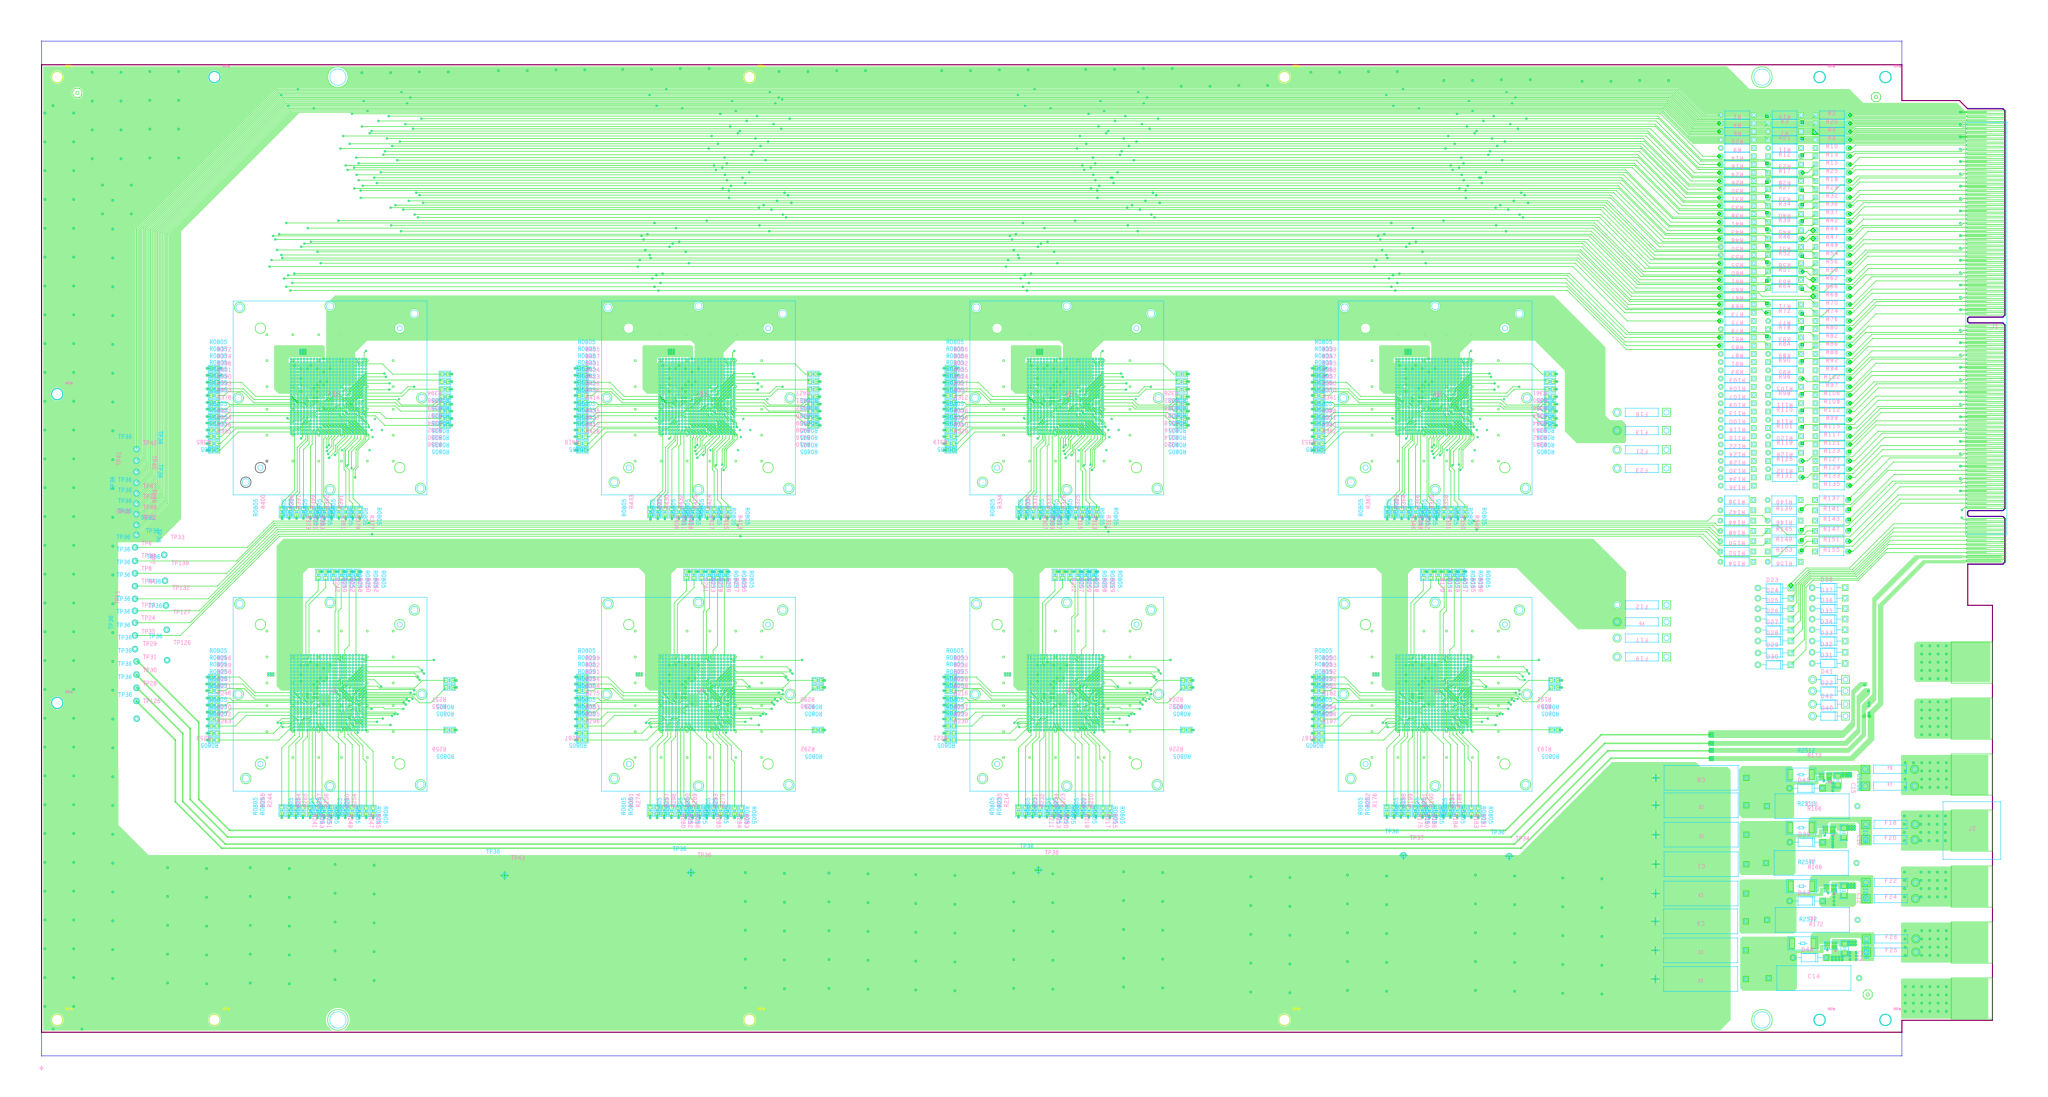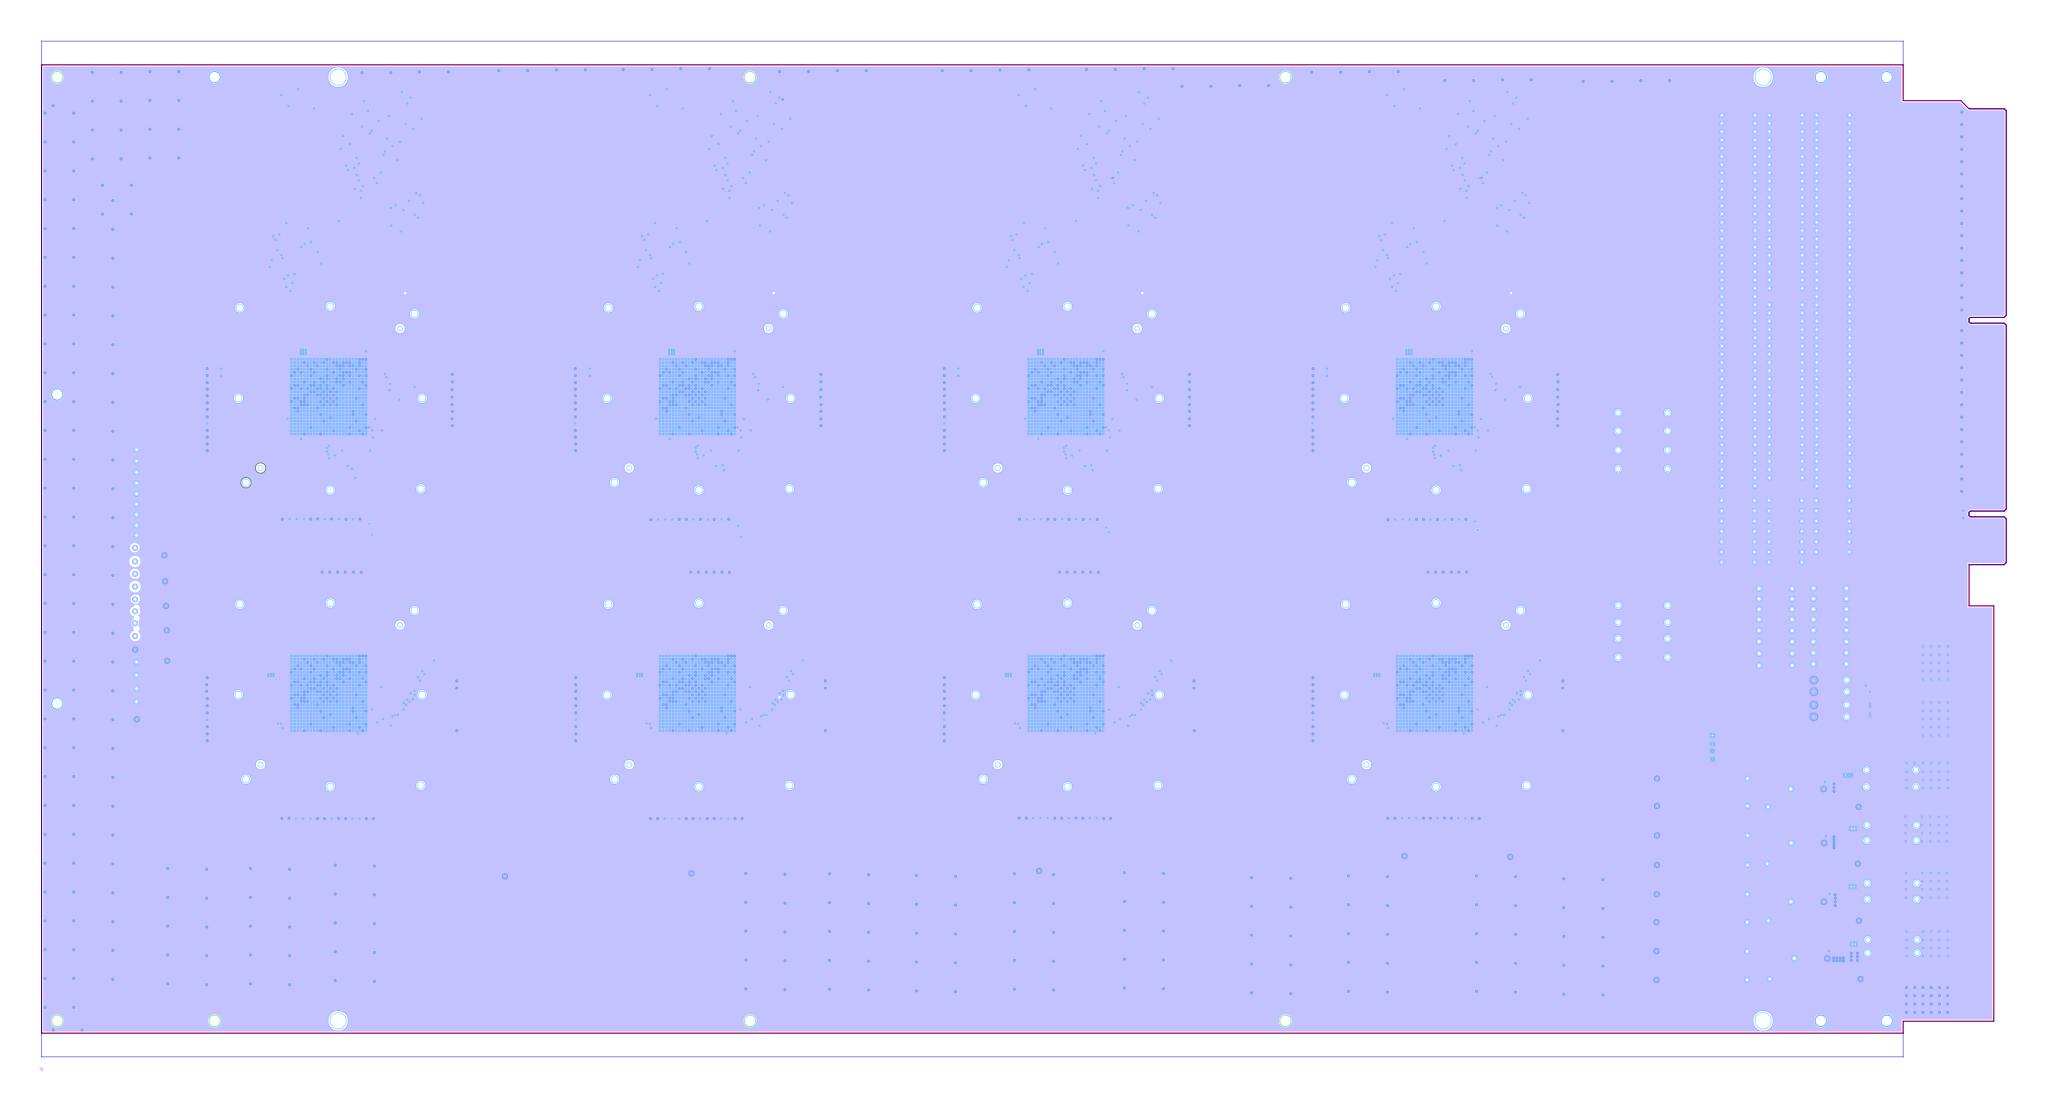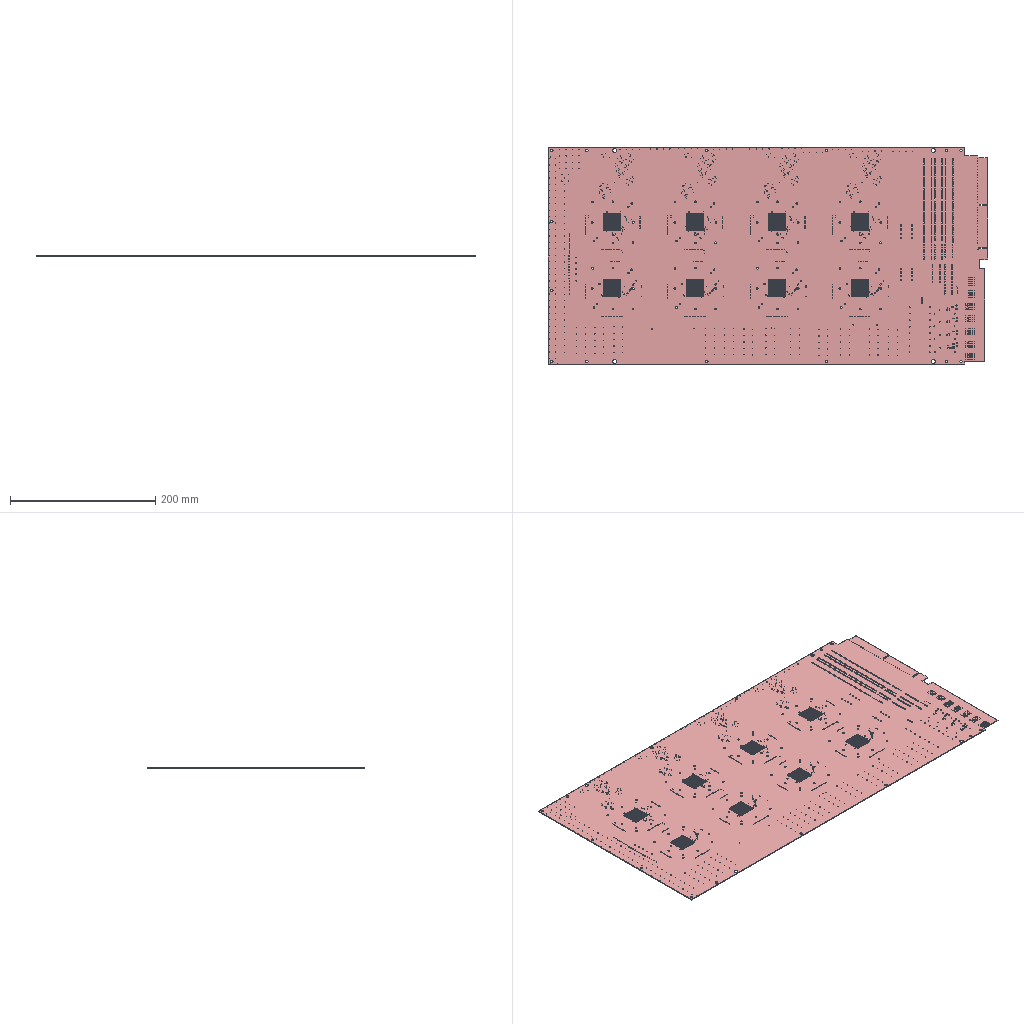Circuit board layout | Cadence Allegro | box 605.8 x 298.4 x 1.1 mm
Layer stack:
# Cadence Allegro layer stack of  (unit mm; from the constraint file cross-section; dielectric type: 0 not recorded (Allegro does not mark core vs prepreg), 3 surface material)
index,name,kind,layer,copper_thickness_mm,dielectric_type,dielectric_thickness_mm,dielectric_material,dielectric_constant
0,Top Surface,other,,,,,,
1,TOP,copper,TOP,0.0305,,,,
2,Dielectric1,dielectric,,,0,0.2032,FR-4,4.5
3,L2_GND,copper,L2_GND,0.0305,,,,
4,Dielectric2,dielectric,,,0,0.2032,FR-4,4.5
5,L3_SIG1,copper,L3_SIG1,0.0305,,,,
6,Dielectric3,dielectric,,,0,0.2032,FR-4,4.5
7,L4_SIG2,copper,L4_SIG2,0.0305,,,,
8,Dielectric4,dielectric,,,0,0.2032,FR-4,4.5
9,L5_POWER,copper,L5_POWER,0.0305,,,,
10,Dielectric5,dielectric,,,0,0.2032,FR-4,4.5
11,BOTTOM,copper,BOTTOM,0.0305,,,,
12,Bottom Surface,other,,,,,,
# drill layer pairs: low layer,high layer
drill_pair,TOP,BOTTOM
Part placement:
REFDES,COMP_VALUE,SYM_NAME,SYM_X,SYM_Y,SYM_ROTATE,SYM_MIRROR
C1,100UF,CAP2-1100,20161.000,2477.000,180.000,NO
C2,100UF,CAP2-1100,20161.000,2836.000,180.000,NO
C3,100UF,CAP2-1100,20158.000,2121.000,180.000,NO
C4,100UF,CAP2-1100,20155.000,1083.000,180.000,NO
C5,100UF,CAP2-1100,20161.000,3193.000,180.000,NO
C6,100UF,CAP2-1100,20155.000,1783.000,180.000,NO
C7,100UF,CAP2-1100,20155.000,1431.000,180.000,NO
C8,100UF,CAP2-1100,20161.000,3526.000,180.000,NO
C9,100UF,CAP2-1100,21499.000,2492.000,0.000,NO
C10,0.1UF,C1206,21895.000,2860.000,270.000,NO
C11,100UF,CAP2-1100,21512.000,1801.000,0.000,NO
C12,0.1UF,C1206,21895.000,2155.000,270.000,NO
C13,0.1UF,C1206,21905.000,1454.000,270.000,NO
C14,100UF,CAP2-1100,21531.000,1094.000,0.000,NO
C15,0.1UF,C1206,21820.000,3494.000,270.000,NO
C16,100UF,CAP2-1100,21509.000,3182.000,0.000,NO
D22,LED,DIODE2-400,21715.000,4580.000,0.000,NO
D23,1N4448,DIODE2-400B,21051.000,5831.000,0.000,NO
D24,1N4448,DIODE2-400B,21051.000,5706.000,0.000,NO
D25,1N4448,DIODE2-400B,21051.000,5581.000,0.000,NO
D26,1N4448,DIODE2-400B,21051.000,5455.000,0.000,NO
D27,1N4448,DIODE2-400B,21051.000,5321.000,0.000,NO
D28,1N4448,DIODE2-400B,21051.000,5189.000,0.000,NO
D29,1N4448,DIODE2-400B,21052.000,5043.000,0.000,NO
D30,1N4448,DIODE2-400B,21051.000,4899.000,0.000,NO
D31,1N4448,DIODE2-400B,21711.000,4916.000,0.000,NO
D32,1N4448,DIODE2-400B,21710.000,5051.000,0.000,NO
D33,1N4448,DIODE2-400B,21711.000,5187.000,0.000,NO
D34,1N4448,DIODE2-400B,21710.000,5325.000,0.000,NO
D35,1N4448,DIODE2-400B,21710.000,5454.000,0.000,NO
D36,1N4448,DIODE2-400B,21712.000,5582.000,0.000,NO
D37,1N4448,DIODE2-400B,21711.000,5708.000,0.000,NO
D38,1N4448,DIODE2-400B,21711.000,5836.000,0.000,NO
D39,BZX79C6V2,DIODE2-400B,21440.000,2744.000,0.000,NO
D40,LED,DIODE2-400,21715.000,4275.000,0.000,NO
D41,LED,DIODE2-400,21715.000,4720.000,0.000,NO
D42,LED,DIODE2-400,21715.000,4420.000,0.000,NO
D43,BZX79C6V2,DIODE2-400B,21437.000,2031.000,0.000,NO
D44,BZX79C6V2,DIODE2-400B,21478.000,1342.000,0.000,NO
D45,BZX79C6V2,DIODE2-400B,21435.000,3400.000,0.000,NO
F7,1A,FU2-600,22455.000,3425.000,0.000,NO
F8,DNP,FU2-600,22455.000,3630.000,0.000,NO
F9,1A,FU2-600,19441.000,5421.000,180.000,NO
F12,1,FU2-600,19441.000,5627.000,180.000,NO
F13,1,FU2-600,19440.000,7744.000,180.000,NO
F16,1,FU2-600,19440.000,7965.000,180.000,NO
F17,1A,FU2-600,19441.000,5224.000,180.000,NO
F18,1A,FU2-600,22462.165,2960.000,0.000,NO
F19,1,FU2-600,19441.000,4996.000,180.000,NO
F20,DNP,FU2-600,22460.000,2775.000,0.000,NO
F21,1,FU2-600,19440.000,7511.000,180.000,NO
F22,1A,FU2-600,22465.000,2255.000,0.000,NO
F23,1,FU2-600,19440.000,7284.000,180.000,NO
F24,DNP,FU2-600,22465.000,2060.000,0.000,NO
F25,1A,FU2-600,22470.000,1410.000,0.000,NO
F26,DNP,FU2-600,22470.000,1570.000,0.000,NO
IC4,INA214,SOP6-26-54,21670.000,3540.000,180.000,NO
J1,FINGER,FINGER,23625.000,8986.417,0.000,NO
J2,FINGER-T,FINGER-T,23450.000,2886.000,0.000,NO
R1,47,RES2-400-100,20600.000,11575.000,180.000,NO
R2,47,RES2-400-100,21750.000,11575.000,0.000,NO
R3,47,RES2-400-100,21175.000,11475.000,0.000,NO
R4,47,RES2-400-100,20600.000,11475.000,180.000,NO
R5,47,RES2-400-100,21750.000,11375.000,0.000,NO
R6,47,RES2-400-100,20600.000,11375.000,180.000,NO
R7,47,RES2-400-100,21175.000,11375.000,180.000,NO
R8,47,RES2-400-100,21750.000,11275.000,0.000,NO
R9,47,RES2-400-100,20600.000,11175.000,180.000,NO
R10,47,RES2-400-100,21750.000,11175.000,0.000,NO
R11,47,RES2-400-100,21175.000,11175.000,180.000,NO
R12,47,RES2-400-100,21175.000,11075.000,0.000,NO
R13,47,RES2-400-100,21750.000,11075.000,0.000,NO
R14,47,RES2-400-100,20600.000,11075.000,180.000,NO
R15,47,RES2-400-100,21750.000,10975.000,0.000,NO
R16,47,RES2-400-100,20600.000,10975.000,180.000,NO
R17,47,RES2-400-100,21175.000,10875.000,0.000,NO
R18,47,RES2-400-100,21750.000,10775.000,0.000,NO
R19,47,RES2-400-100,21175.000,11575.000,180.000,NO
R20,47,RES2-400-100,21750.000,11475.000,0.000,NO
R21,47,RES2-400-100,21175.000,11275.000,0.000,NO
R22,47,RES2-400-100,20600.000,11275.000,180.000,NO
R23,47,RES2-400-100,21175.000,10975.000,180.000,NO
R24,47,RES2-400-100,20600.000,10875.000,180.000,NO
R25,47,RES2-400-100,21750.000,10875.000,0.000,NO
R26,47,RES2-400-100,20600.000,10775.000,180.000,NO
R27,47,RES2-400-100,21175.000,10675.000,0.000,NO
R28,47,RES2-400-100,21175.000,10775.000,180.000,NO
R29,47,RES2-400-100,21750.000,10675.000,0.000,NO
R30,47,RES2-400-100,20600.000,10675.000,180.000,NO
R31,47,RES2-400-100,20600.000,10575.000,180.000,NO
R32,47,RES2-400-100,21750.000,10575.000,0.000,NO
R33,47,RES2-400-100,21175.000,10575.000,180.000,NO
R34,47,RES2-400-100,21175.000,10475.000,0.000,NO
R35,47,RES2-400-100,20600.000,10475.000,180.000,NO
R36,47,RES2-400-100,21750.000,10475.000,0.000,NO
R37,47,RES2-400-100,21750.000,10375.000,0.000,NO
R38,47,RES2-400-100,20600.000,10375.000,180.000,NO
R39,47,RES2-400-100,21175.000,10275.000,0.000,NO
R40,47,RES2-400-100,21175.000,10375.000,180.000,NO
R41,47,RES2-400-100,20600.000,10275.000,180.000,NO
R42,47,RES2-400-100,21750.000,10275.000,0.000,NO
R43,47,RES2-400-100,20600.000,10175.000,180.000,NO
R44,47,RES2-400-100,21750.000,10175.000,0.000,NO
R45,47,RES2-400-100,21175.000,10175.000,180.000,NO
R46,47,RES2-400-100,21175.000,10075.000,0.000,NO
R47,47,RES2-400-100,21750.000,10075.000,0.000,NO
R48,47,RES2-400-100,20600.000,10075.000,180.000,NO
R49,47,RES2-400-100,21750.000,9975.000,0.000,NO
R50,47,RES2-400-100,20600.000,9975.000,180.000,NO
R51,47,RES2-400-100,21175.000,9975.000,180.000,NO
R52,47,RES2-400-100,21175.000,9875.000,0.000,NO
R53,47,RES2-400-100,20600.000,9875.000,180.000,NO
R54,47,RES2-400-100,21750.000,9875.000,0.000,NO
R55,47,RES2-400-100,20600.000,9775.000,180.000,NO
R56,47,RES2-400-100,21750.000,9775.000,0.000,NO
R57,47,RES2-400-100,21175.000,9675.000,0.000,NO
R58,47,RES2-400-100,21175.000,9775.000,180.000,NO
R59,47,RES2-400-100,21750.000,9675.000,0.000,NO
R60,47,RES2-400-100,20600.000,9675.000,180.000,NO
R61,47,RES2-400-100,20600.000,9575.000,180.000,NO
R62,47,RES2-400-100,21750.000,9575.000,0.000,NO
R63,47,RES2-400-100,21175.000,9575.000,180.000,NO
R64,47,RES2-400-100,21175.000,9475.000,0.000,NO
R65,47,RES2-400-100,20600.000,9475.000,180.000,NO
R66,47,RES2-400-100,21750.000,9475.000,0.000,NO
R67,47,RES2-400-100,20600.000,9375.000,180.000,NO
R68,47,RES2-400-100,21750.000,9375.000,0.000,NO
R69,47,RES2-400-100,20600.000,9275.000,180.000,NO
R70,47,RES2-400-100,21750.000,9275.000,0.000,NO
R71,47,RES2-400-100,21175.000,9275.000,180.000,NO
R72,47,RES2-400-100,21175.000,9175.000,0.000,NO
R73,47,RES2-400-100,20600.000,9175.000,180.000,NO
R74,47,RES2-400-100,21750.000,9175.000,0.000,NO
R75,47,RES2-400-100,20600.000,9075.000,180.000,NO
R76,47,RES2-400-100,21750.000,9075.000,0.000,NO
R77,47,RES2-400-100,21175.000,9075.000,180.000,NO
R78,47,RES2-400-100,21175.000,8975.000,0.000,NO
R79,47,RES2-400-100,20600.000,8975.000,180.000,NO
R80,47,RES2-400-100,21750.000,8975.000,0.000,NO
R81,47,RES2-400-100,20600.000,8875.000,180.000,NO
R82,47,RES2-400-100,21750.000,8875.000,0.000,NO
R83,47,RES2-400-100,21175.000,8875.000,180.000,NO
R84,47,RES2-400-100,21175.000,8775.000,0.000,NO
R85,47,RES2-400-100,20600.000,8775.000,180.000,NO
R86,47,RES2-400-100,21750.000,8775.000,0.000,NO
R87,47,RES2-400-100,20600.000,8675.000,180.000,NO
R88,47,RES2-400-100,21750.000,8675.000,0.000,NO
R89,47,RES2-400-100,21175.000,8675.000,180.000,NO
R90,47,RES2-400-100,21175.000,8575.000,0.000,NO
R91,47,RES2-400-100,20600.000,8575.000,180.000,NO
R92,47,RES2-400-100,21750.000,8575.000,0.000,NO
R93,47,RES2-400-100,20600.000,8475.000,180.000,NO
R94,47,RES2-400-100,21750.000,8475.000,0.000,NO
R95,47,RES2-400-100,21175.000,8475.000,180.000,NO
R96,47,RES2-400-100,21175.000,8375.000,0.000,NO
R97,100,RES2-400-100,21750.000,8275.000,0.000,NO
R98,100,RES2-400-100,21175.000,8175.000,0.000,NO
R99,100,RES2-400-100,21750.000,7875.000,0.000,NO
R100,100,RES2-400-100,20600.000,7875.000,180.000,NO
R101,100,RES2-400-100,21175.000,7775.000,0.000,NO
R102,100,RES2-400-100,21750.000,8375.000,0.000,NO
R103,100,RES2-400-100,20600.000,8375.000,180.000,NO
R104,100,RES2-400-100,20600.000,8275.000,180.000,NO
R105,100,RES2-400-100,21175.000,8275.000,180.000,NO
R106,100,RES2-400-100,21750.000,8175.000,0.000,NO
R107,100,RES2-400-100,20600.000,8175.000,180.000,NO
R108,100,RES2-400-100,21750.000,8075.000,0.000,NO
R109,100,RES2-400-100,20600.000,8075.000,180.000,NO
R110,100,RES2-400-100,21175.000,7975.000,0.000,NO
R111,100,RES2-400-100,21175.000,8075.000,180.000,NO
R112,100,RES2-400-100,21750.000,7975.000,0.000,NO
R113,100,RES2-400-100,20600.000,7975.000,180.000,NO
R114,100,RES2-400-100,21175.000,7875.000,180.000,NO
R115,100,RES2-400-100,21750.000,7775.000,0.000,NO
R116,100,RES2-400-100,20600.000,7775.000,180.000,NO
R117,100,RES2-400-100,21750.000,7675.000,0.000,NO
R118,100,RES2-400-100,20600.000,7675.000,180.000,NO
R119,100,RES2-400-100,21175.000,7575.000,0.000,NO
R120,100,RES2-400-100,21175.000,7675.000,180.000,NO
R121,100,RES2-400-100,21750.000,7575.000,0.000,NO
R122,100,RES2-400-100,20600.000,7575.000,180.000,NO
R123,100,RES2-400-100,21750.000,7475.000,0.000,NO
R124,100,RES2-400-100,20600.000,7475.000,180.000,NO
R125,100,RES2-400-100,21175.000,7375.000,0.000,NO
R126,100,RES2-400-100,21175.000,7475.000,180.000,NO
R127,100,RES2-400-100,21750.000,7375.000,0.000,NO
R128,100,RES2-400-100,20600.000,7375.000,180.000,NO
R129,100,RES2-400-100,21750.000,7275.000,0.000,NO
R130,100,RES2-400-100,20600.000,7275.000,180.000,NO
R131,100,RES2-400-100,21175.000,7175.000,0.000,NO
R132,100,RES2-400-100,21175.000,7275.000,180.000,NO
R133,100,RES2-400-100,21750.000,7175.000,0.000,NO
R134,100,RES2-400-100,20600.000,7175.000,180.000,NO
R135,100,RES2-400-100,21750.000,7075.000,0.000,NO
R136,100,RES2-400-100,20600.000,7075.000,180.000,NO
R137,100,RES2-400-100,21745.000,6900.000,0.000,NO
R138,100,RES2-400-100,20595.000,6900.000,180.000,NO
R139,100,RES2-400-100,21170.000,6775.000,0.000,NO
R140,100,RES2-400-100,21170.000,6900.000,180.000,NO
R141,100,RES2-400-100,21745.000,6775.000,0.000,NO
R142,100,RES2-400-100,20595.000,6775.000,180.000,NO
R143,100,RES2-400-100,21745.000,6650.000,0.000,NO
R144,100,RES2-400-100,20595.000,6650.000,180.000,NO
R145,100,RES2-400-100,21170.000,6525.000,0.000,NO
R146,100,RES2-400-100,21170.000,6650.000,180.000,NO
R147,100,RES2-400-100,21745.000,6525.000,0.000,NO
R148,100,RES2-400-100,20595.000,6525.000,180.000,NO
R149,100,RES2-400-100,21170.000,6400.000,0.000,NO
R150,100,RES2-400-100,20595.000,6400.000,180.000,NO
R151,100,RES2-400-100,21745.000,6400.000,0.000,NO
R152,100,RES2-400-100,20595.000,6275.000,180.000,NO
R153,100,RES2-400-100,21170.000,6275.000,0.000,NO
R154,100,RES2-400-100,20595.000,6150.000,180.000,NO
R155,100,RES2-400-100,21745.000,6275.000,0.000,NO
R156,100,RES2-400-100,21170.000,6150.000,180.000,NO
R166,0.010R/2W,R2512,21375.000,2920.000,0.000,NO
R167,332R,R0805,22100.000,4275.000,0.000,YES
R168,0.010R/2W,R2512,21380.000,2210.000,0.000,NO
R169,332R,R0805,22120.000,4720.000,0.000,YES
R170,332R,R0805,22095.000,4420.000,0.000,YES
R171,332R,R0805,22110.000,4580.000,0.000,YES
R172,0.010R/2W,R2512,21396.000,1516.000,0.000,NO
R173,0.010R/2W,R2512,21375.000,3565.000,0.000,NO
R174,4.7K,R0805,16877.000,5991.000,270.000,NO
R175,4.7K,R0805,16514.000,3127.000,270.000,NO
R176,4.7K,R0805,16429.000,3128.000,90.000,NO
R177,4.7K,R0805,17065.000,5991.000,270.000,NO
R178,4.7K,R0805,16970.000,5991.000,270.000,NO
R179,4.7K,R0805,16786.000,5991.000,270.000,NO
R180,4.7K,R0805,16601.000,3127.000,270.000,NO
R181,4.7K,R0805,17285.000,3126.000,270.000,NO
R182,4.7K,R0805,15520.000,4324.000,0.000,NO
R183,4.7K,R0805,17199.000,3127.000,270.000,NO
R184,4.7K,R0805,16946.000,3128.000,270.000,NO
R185,4.7K,R0805,17162.000,5991.000,270.000,NO
R186,4.7K,R0805,16689.000,3125.000,270.000,NO
R187,4.7K,R0805,15518.000,4240.000,180.000,NO
R188,4.7K,R0805,17453.000,3124.000,90.000,NO
R189,4.7K,R0805,18380.000,4624.000,180.000,NO
R190,4.7K,R0805,17115.000,3128.000,90.000,NO
R191,4.7K,R0805,18380.000,4710.000,180.000,NO
R192,4.7K,R0805,15520.000,4585.000,0.000,NO
R193,4.7K,R0805,18382.000,4107.000,180.000,NO
R194,4.7K,R0805,17369.000,3124.000,90.000,NO
R195,4.7K,R0805,15520.000,4495.000,0.000,NO
R196,4.7K,R0805,17252.000,5992.000,270.000,NO
R197,4.7K,R0805,15520.000,3985.000,0.000,NO
R198,4.7K,R0805,16776.000,3127.000,90.000,NO
R199,4.7K,R0805,16860.000,3126.000,90.000,NO
R200,4.7K,R0805,15520.000,4750.000,0.000,NO
R201,4.7K,R0805,17032.000,3128.000,90.000,NO
R202,4.7K,R0805,16343.000,3130.000,90.000,NO
R203,4.7K,R0805,15520.000,4665.000,0.000,NO
R204,4.7K,R0805,15520.000,4155.000,0.000,NO
R205,4.7K,R0805,15520.000,4410.000,0.000,NO
R206,4.7K,R0805,15520.000,4068.000,0.000,NO
R207,4.7K,R0805,12402.000,5991.000,270.000,NO
R208,4.7K,R0805,12687.000,5991.000,270.000,NO
R209,4.7K,R0805,12495.000,5991.000,270.000,NO
R210,4.7K,R0805,12978.000,3124.000,90.000,NO
R211,4.7K,R0805,12039.000,3127.000,270.000,NO
R212,4.7K,R0805,12311.000,5991.000,270.000,NO
R213,4.7K,R0805,12126.000,3127.000,270.000,NO
R214,4.7K,R0805,11954.000,3128.000,90.000,NO
R215,4.7K,R0805,12810.000,3126.000,270.000,NO
R216,4.7K,R0805,11045.000,4324.000,0.000,NO
R217,4.7K,R0805,12724.000,3127.000,270.000,NO
R218,4.7K,R0805,12590.000,5991.000,270.000,NO
R219,4.7K,R0805,12471.000,3128.000,270.000,NO
R220,4.7K,R0805,12214.000,3125.000,270.000,NO
R221,4.7K,R0805,11043.000,4240.000,180.000,NO
R222,4.7K,R0805,13905.000,4624.000,180.000,NO
R223,4.7K,R0805,12640.000,3128.000,90.000,NO
R224,4.7K,R0805,13905.000,4710.000,180.000,NO
R225,4.7K,R0805,11045.000,4585.000,0.000,NO
R226,4.7K,R0805,13907.000,4107.000,180.000,NO
R227,4.7K,R0805,12894.000,3124.000,90.000,NO
R228,4.7K,R0805,11045.000,4495.000,0.000,NO
R229,4.7K,R0805,12781.000,5990.000,270.000,NO
R230,4.7K,R0805,11045.000,3985.000,0.000,NO
R231,4.7K,R0805,12301.000,3127.000,90.000,NO
R232,4.7K,R0805,12385.000,3126.000,90.000,NO
R233,4.7K,R0805,11045.000,4750.000,0.000,NO
R234,4.7K,R0805,12557.000,3128.000,90.000,NO
R235,4.7K,R0805,11868.000,3130.000,90.000,NO
R236,4.7K,R0805,11045.000,4665.000,0.000,NO
R237,4.7K,R0805,11045.000,4155.000,0.000,NO
R238,4.7K,R0805,11045.000,4410.000,0.000,NO
R239,4.7K,R0805,11045.000,4068.000,0.000,NO
R240,4.7K,R0805,3452.000,5991.000,270.000,NO
R241,4.7K,R0805,3089.000,3127.000,270.000,NO
R242,4.7K,R0805,3361.000,5991.000,270.000,NO
R243,4.7K,R0805,3176.000,3127.000,270.000,NO
R244,4.7K,R0805,3004.000,3128.000,90.000,NO
R245,4.7K,R0805,3860.000,3126.000,270.000,NO
R246,4.7K,R0805,2095.000,4324.000,0.000,NO
R247,4.7K,R0805,3774.000,3127.000,270.000,NO
R248,4.7K,R0805,3640.000,5991.000,270.000,NO
R249,4.7K,R0805,3521.000,3128.000,270.000,NO
R250,4.7K,R0805,3737.000,5991.000,270.000,NO
R251,4.7K,R0805,3264.000,3125.000,270.000,NO
R252,4.7K,R0805,3545.000,5991.000,270.000,NO
R253,4.7K,R0805,2093.000,4240.000,180.000,NO
R254,4.7K,R0805,4028.000,3124.000,90.000,NO
R255,4.7K,R0805,4955.000,4624.000,180.000,NO
R256,4.7K,R0805,3690.000,3128.000,90.000,NO
R257,4.7K,R0805,4955.000,4710.000,180.000,NO
R258,4.7K,R0805,2095.000,4585.000,0.000,NO
R259,4.7K,R0805,4957.000,4107.000,180.000,NO
R260,4.7K,R0805,3944.000,3124.000,90.000,NO
R261,4.7K,R0805,2095.000,4495.000,0.000,NO
R262,4.7K,R0805,3835.000,5990.000,270.000,NO
R263,4.7K,R0805,2095.000,3985.000,0.000,NO
R264,4.7K,R0805,3351.000,3127.000,90.000,NO
R265,4.7K,R0805,3435.000,3126.000,90.000,NO
R266,4.7K,R0805,2095.000,4750.000,0.000,NO
R267,4.7K,R0805,3607.000,3128.000,90.000,NO
R268,4.7K,R0805,2918.000,3130.000,90.000,NO
R269,4.7K,R0805,2095.000,4665.000,0.000,NO
R270,4.7K,R0805,2095.000,4155.000,0.000,NO
R271,4.7K,R0805,2095.000,4410.000,0.000,NO
R272,4.7K,R0805,2095.000,4068.000,0.000,NO
R273,4.7K,R0805,7927.000,5991.000,270.000,NO
R274,4.7K,R0805,7479.000,3128.000,90.000,NO
R275,4.7K,R0805,6570.000,4324.000,0.000,NO
R276,4.7K,R0805,8115.000,5991.000,270.000,NO
R277,4.7K,R0805,8212.000,5991.000,270.000,NO
R278,4.7K,R0805,8020.000,5991.000,270.000,NO
R279,4.7K,R0805,8503.000,3124.000,90.000,NO
R280,4.7K,R0805,7564.000,3127.000,270.000,NO
R281,4.7K,R0805,7836.000,5991.000,270.000,NO
R282,4.7K,R0805,7651.000,3127.000,270.000,NO
R283,4.7K,R0805,8335.000,3126.000,270.000,NO
R284,4.7K,R0805,8249.000,3127.000,270.000,NO
R285,4.7K,R0805,7996.000,3128.000,270.000,NO
R286,4.7K,R0805,7739.000,3125.000,270.000,NO
R287,4.7K,R0805,6568.000,4240.000,180.000,NO
R288,4.7K,R0805,9430.000,4624.000,180.000,NO
R289,4.7K,R0805,8165.000,3128.000,90.000,NO
R290,4.7K,R0805,9430.000,4710.000,180.000,NO
R291,4.7K,R0805,6570.000,4585.000,0.000,NO
R292,4.7K,R0805,9432.000,4107.000,180.000,NO
R293,4.7K,R0805,8419.000,3124.000,90.000,NO
R294,4.7K,R0805,6570.000,4495.000,0.000,NO
R295,4.7K,R0805,8305.000,5990.000,270.000,NO
R296,4.7K,R0805,6570.000,3985.000,0.000,NO
R297,4.7K,R0805,7826.000,3127.000,90.000,NO
R298,4.7K,R0805,7910.000,3126.000,90.000,NO
R299,4.7K,R0805,6570.000,4750.000,0.000,NO
R300,4.7K,R0805,8082.000,3128.000,90.000,NO
R301,4.7K,R0805,7393.000,3130.000,90.000,NO
R302,4.7K,R0805,6570.000,4665.000,0.000,NO
R303,4.7K,R0805,6570.000,4155.000,0.000,NO
R304,4.7K,R0805,6570.000,4410.000,0.000,NO
R305,4.7K,R0805,6570.000,4068.000,0.000,NO
R306,4.7K,R0805,11045.000,8500.000,0.000,NO
R307,4.7K,R0805,11960.000,6752.000,270.000,NO
R308,4.7K,R0805,11045.000,8415.000,0.000,NO
R309,4.7K,R0805,12047.000,6752.000,270.000,NO
R310,4.7K,R0805,11045.000,7585.000,0.000,NO
R311,4.7K,R0805,12731.000,6755.000,270.000,NO
R312,4.7K,R0805,11045.000,7915.000,0.000,NO
R313,4.7K,R0805,12562.000,6753.000,270.000,NO
R314,4.7K,R0805,13850.000,7891.000,180.000,NO
R315,4.7K,R0805,12387.000,6753.000,270.000,NO
R316,4.7K,R0805,13850.000,7980.000,180.000,NO
R317,4.7K,R0805,12132.000,6753.000,270.000,NO
R318,4.7K,R0805,13850.000,8064.000,180.000,NO
R319,4.7K,R0805,11043.000,7835.000,180.000,NO
R320,4.7K,R0805,13850.000,7807.000,180.000,NO
R321,4.7K,R0805,13850.000,8154.000,180.000,NO
R322,4.7K,R0805,13850.000,8339.000,180.000,NO
R323,4.7K,R0805,13850.000,8246.000,180.000,NO
R324,4.7K,R0805,11045.000,8170.000,0.000,NO
R325,4.7K,R0805,12816.000,6754.000,90.000,NO
R326,4.7K,R0805,12646.000,6754.000,90.000,NO
R327,4.7K,R0805,11045.000,8085.000,0.000,NO
R328,4.7K,R0805,13850.000,8430.000,180.000,NO
R329,4.7K,R0805,11045.000,7505.000,0.000,NO
R330,4.7K,R0805,12217.000,6755.000,90.000,NO
R331,4.7K,R0805,12302.000,6755.000,90.000,NO
R332,4.7K,R0805,11045.000,8330.000,0.000,NO
R333,4.7K,R0805,12472.000,6755.000,90.000,NO
R334,4.7K,R0805,11872.000,6755.000,90.000,NO
R335,4.7K,R0805,11045.000,8250.000,0.000,NO
R336,4.7K,R0805,11045.000,7750.000,0.000,NO
R337,4.7K,R0805,11045.000,8005.000,0.000,NO
R338,4.7K,R0805,11045.000,7670.000,0.000,NO
R339,4.7K,R0805,15520.000,8500.000,0.000,NO
R340,4.7K,R0805,15520.000,7585.000,0.000,NO
R341,4.7K,R0805,15520.000,7915.000,0.000,NO
R342,4.7K,R0805,18325.000,7891.000,180.000,NO
R343,4.7K,R0805,18325.000,7980.000,180.000,NO
R344,4.7K,R0805,18325.000,8064.000,180.000,NO
R345,4.7K,R0805,18325.000,7807.000,180.000,NO
R346,4.7K,R0805,16435.000,6752.000,270.000,NO
R347,4.7K,R0805,15520.000,8415.000,0.000,NO
R348,4.7K,R0805,16522.000,6752.000,270.000,NO
R349,4.7K,R0805,17206.000,6755.000,270.000,NO
R350,4.7K,R0805,17037.000,6753.000,270.000,NO
R351,4.7K,R0805,16862.000,6753.000,270.000,NO
R352,4.7K,R0805,16607.000,6753.000,270.000,NO
R353,4.7K,R0805,15518.000,7835.000,180.000,NO
R354,4.7K,R0805,18325.000,8154.000,180.000,NO
R355,4.7K,R0805,18325.000,8339.000,180.000,NO
R356,4.7K,R0805,18325.000,8246.000,180.000,NO
R357,4.7K,R0805,15520.000,8170.000,0.000,NO
R358,4.7K,R0805,17291.000,6754.000,90.000,NO
R359,4.7K,R0805,17121.000,6754.000,90.000,NO
R360,4.7K,R0805,15520.000,8085.000,0.000,NO
R361,4.7K,R0805,18325.000,8430.000,180.000,NO
R362,4.7K,R0805,15520.000,7505.000,0.000,NO
R363,4.7K,R0805,16692.000,6755.000,90.000,NO
R364,4.7K,R0805,16777.000,6755.000,90.000,NO
R365,4.7K,R0805,15520.000,8330.000,0.000,NO
R366,4.7K,R0805,16947.000,6755.000,90.000,NO
R367,4.7K,R0805,16347.000,6755.000,90.000,NO
R368,4.7K,R0805,15520.000,8250.000,0.000,NO
R369,4.7K,R0805,15520.000,7750.000,0.000,NO
R370,4.7K,R0805,15520.000,8005.000,0.000,NO
R371,4.7K,R0805,15520.000,7670.000,0.000,NO
R372,4.7K,R0805,2095.000,8500.000,0.000,NO
R373,4.7K,R0805,3010.000,6752.000,270.000,NO
R374,4.7K,R0805,2095.000,8415.000,0.000,NO
R375,4.7K,R0805,3097.000,6752.000,270.000,NO
R376,4.7K,R0805,2095.000,7585.000,0.000,NO
R377,4.7K,R0805,3781.000,6755.000,270.000,NO
R378,4.7K,R0805,2095.000,7915.000,0.000,NO
R379,4.7K,R0805,3612.000,6753.000,270.000,NO
R380,4.7K,R0805,4900.000,7891.000,180.000,NO
R381,4.7K,R0805,3437.000,6753.000,270.000,NO
R382,4.7K,R0805,4900.000,7980.000,180.000,NO
R383,4.7K,R0805,3182.000,6753.000,270.000,NO
R384,4.7K,R0805,4900.000,8064.000,180.000,NO
R385,4.7K,R0805,2093.000,7835.000,180.000,NO
R386,4.7K,R0805,4900.000,7807.000,180.000,NO
R387,4.7K,R0805,4900.000,8154.000,180.000,NO
R388,4.7K,R0805,4900.000,8339.000,180.000,NO
R389,4.7K,R0805,4900.000,8246.000,180.000,NO
R390,4.7K,R0805,2095.000,8170.000,0.000,NO
R391,4.7K,R0805,3866.000,6754.000,90.000,NO
R392,4.7K,R0805,3696.000,6754.000,90.000,NO
R393,4.7K,R0805,2095.000,8085.000,0.000,NO
R394,4.7K,R0805,4900.000,8430.000,180.000,NO
R395,4.7K,R0805,2095.000,7505.000,0.000,NO
R396,4.7K,R0805,3267.000,6755.000,90.000,NO
R397,4.7K,R0805,3352.000,6755.000,90.000,NO
R398,4.7K,R0805,2095.000,8330.000,0.000,NO
R399,4.7K,R0805,3522.000,6755.000,90.000,NO
R400,4.7K,R0805,2922.000,6755.000,90.000,NO
R401,4.7K,R0805,2095.000,8250.000,0.000,NO
R402,4.7K,R0805,2095.000,7750.000,0.000,NO
R403,4.7K,R0805,2095.000,8005.000,0.000,NO
R404,4.7K,R0805,2095.000,7670.000,0.000,NO
R405,4.7K,R0805,6570.000,8500.000,0.000,NO
R406,4.7K,R0805,7485.000,6752.000,270.000,NO
R407,4.7K,R0805,6570.000,8415.000,0.000,NO
R408,4.7K,R0805,9375.000,7980.000,180.000,NO
R409,4.7K,R0805,9375.000,8064.000,180.000,NO
R410,4.7K,R0805,9375.000,7807.000,180.000,NO
R411,4.7K,R0805,7572.000,6752.000,270.000,NO
R412,4.7K,R0805,6570.000,7585.000,0.000,NO
R413,4.7K,R0805,8256.000,6755.000,270.000,NO
R414,4.7K,R0805,6570.000,7915.000,0.000,NO
R415,4.7K,R0805,8087.000,6753.000,270.000,NO
R416,4.7K,R0805,9375.000,7891.000,180.000,NO
R417,4.7K,R0805,7912.000,6753.000,270.000,NO
R418,4.7K,R0805,7657.000,6753.000,270.000,NO
R419,4.7K,R0805,6568.000,7835.000,180.000,NO
R420,4.7K,R0805,9375.000,8154.000,180.000,NO
R421,4.7K,R0805,9375.000,8339.000,180.000,NO
R422,4.7K,R0805,9375.000,8246.000,180.000,NO
R423,4.7K,R0805,6570.000,8170.000,0.000,NO
R424,4.7K,R0805,8341.000,6754.000,90.000,NO
R425,4.7K,R0805,8171.000,6754.000,90.000,NO
R426,4.7K,R0805,6570.000,8085.000,0.000,NO
R427,4.7K,R0805,9375.000,8430.000,180.000,NO
R428,4.7K,R0805,6570.000,7505.000,0.000,NO
R429,4.7K,R0805,7742.000,6755.000,90.000,NO
R430,4.7K,R0805,7827.000,6755.000,90.000,NO
R431,4.7K,R0805,6570.000,8330.000,0.000,NO
R432,4.7K,R0805,7997.000,6755.000,90.000,NO
R433,4.7K,R0805,7397.000,6755.000,90.000,NO
R434,4.7K,R0805,6570.000,8250.000,0.000,NO
R435,4.7K,R0805,6570.000,7750.000,0.000,NO
R436,4.7K,R0805,6570.000,8005.000,0.000,NO
R437,4.7K,R0805,6570.000,7670.000,0.000,NO
TP6,TPT,TP36,1135.000,6160.000,0.000,NO
TP7,TPT,TP36,1135.000,6325.000,270.000,NO
TP8,TPT,TP36,1135.000,5855.000,0.000,NO
TP11,TPT,TP36,1135.000,5555.000,90.000,NO
TP21,TPT,TP36,1153.000,6729.000,0.000,NO
TP22,TPT,TP36,1153.000,6477.000,0.000,NO
TP23,TPT,TP36,1135.000,5410.000,0.000,NO
TP24,TPT,TP36,1135.000,5255.000,0.000,NO
TP28,TPT,TP36,1153.000,4460.000,0.000,NO
TP29,TPT,TP36,1153.000,4940.000,0.000,NO
TP30,TPT,TP36,1153.000,4620.000,0.000,NO
TP31,TPT,TP36,1153.000,4780.000,0.000,NO
TP33,TPT,TP36,1490.000,6235.000,0.000,NO
TP34,TPT,TP36,17830.000,2575.000,0.000,NO
TP35,TPT,TP36,1135.000,5090.000,0.000,NO
TP36,TPT,TP36,7890.000,2375.000,0.000,NO
TP37,TPT,TP36,16545.000,2585.000,0.000,NO
TP38,TPT,TP36,12110.000,2405.000,0.000,NO
TP39,TPT,TP36,1135.000,6010.000,0.000,NO
TP40,TPT,TP36,1153.000,7518.000,270.000,NO
TP41,TPT,TP36,1153.000,7242.000,90.000,NO
TP42,TPT,TP36,1153.000,7379.000,0.000,NO
TP43,TPT,TP36,5625.000,2340.000,0.000,NO
TP44,TPT,TP36,1135.000,5700.000,0.000,NO
TP45,TPT,TP36,1153.000,6981.000,180.000,NO
TP46,TPT,TP36,1153.000,7111.000,270.000,NO
TP47,TPT,TP36,1153.000,6855.000,0.000,NO
TP48,TPT,TP36,1153.000,6598.000,0.000,NO
TP125,TPT,TP36,1155.000,4245.000,0.000,NO
TP126,TPT,TP36,1525.000,4955.000,0.000,NO
TP127,TPT,TP36,1520.000,5325.000,0.000,NO
TP132,TPT,TP36,1510.000,5620.000,0.000,NO
TP139,TPT,TP36,1500.000,5920.000,0.000,NO
U1,SOCKET_ZXC190,BGA-576,16930.000,4541.000,0.000,NO
U2,SOCKET_ZXC190,BGA-576,12455.000,4541.000,0.000,NO
U3,SOCKET_ZXC190,BGA-576,3505.000,4541.000,0.000,NO
U4,SOCKET_ZXC190,BGA-576,7980.000,4541.000,0.000,NO
U5,SOCKET_ZXC190,BGA-576,12455.000,8140.000,0.000,NO
U6,SOCKET_ZXC190,BGA-576,16930.000,8140.000,0.000,NO
U7,INA214,SOP6-26-54,21715.000,2895.000,180.000,NO
U8,INA214,SOP6-26-54,21730.000,2185.000,180.000,NO
U9,INA214,SOP6-26-54,21736.000,1489.000,180.000,NO
U10,SOCKET_ZXC190,BGA-576,3505.000,8140.000,0.000,NO
U11,SOCKET_ZXC190,BGA-576,7980.000,8140.000,0.000,NO
Pad and via stacks:
# Allegro (Cadence) via spans and padstacks; design units: ("mils" 3 1000)
# via spans: padstack,start_layer,end_layer,net_example,count
VIA12_GEN,ETCH/TOP,ETCH/BOTTOM,GND,733
VIA20D10,ETCH/TOP,ETCH/BOTTOM,VCC_3.3V(ROW1),641
# Allegro padstack definitions: name,start_layer,end_layer,drill,plating,holeType,type
ID-BOARD,"ETCH/TOP","ETCH/TOP",0.0,"PLATED","none","smd"
SMD115_30,"ETCH/TOP","ETCH/TOP",0.0,"NON_PLATED","none","smd"
SMD100_22,"ETCH/TOP","ETCH/TOP",0.0,"PLATED","none","smd"
SMD45_22,"ETCH/TOP","ETCH/TOP",0.0,"PLATED","none","smd"
SMD15_80,"ETCH/TOP","ETCH/TOP",0.0,"NON_PLATED","none","smd"
SMD15_32,"ETCH/TOP","ETCH/TOP",0.0,"NON_PLATED","none","smd"
BALL12,"ETCH/TOP","ETCH/TOP",0.0,"PLATED","none","smd"
SMD55_65,"ETCH/TOP","ETCH/TOP",0.0,"PLATED","none","smd"
SMD480_30_B,"ETCH/BOTTOM","ETCH/BOTTOM",0.0,"NON_PLATED","none","smd"
SMD480_30,"ETCH/TOP","ETCH/TOP",0.0,"NON_PLATED","none","smd"
SMD500SQ_B,"ETCH/BOTTOM","ETCH/BOTTOM",0.0,"PLATED","none","smd"
SMD500SQ,"ETCH/TOP","ETCH/TOP",0.0,"PLATED","none","smd"
SMD50_15,"ETCH/TOP","ETCH/TOP",0.0,"NON_PLATED","none","smd"
SMD60_125,"ETCH/TOP","ETCH/TOP",0.0,"PLATED","none","smd"
SMD40_45,"ETCH/TOP","ETCH/TOP",0.0,"PLATED","none","smd"
SMD45_50,"ETCH/TOP","ETCH/TOP",0.0,"PLATED","none","smd"
Y33,"ETCH/TOP","ETCH/TOP",0.0,"NON_PLATED","none","smd"
Y6,"ETCH/TOP","ETCH/TOP",0.0,"NON_PLATED","none","smd"
Y4,"ETCH/TOP","ETCH/TOP",0.0,"NON_PLATED","none","smd"
PAD70CIR47D,"ETCH/TOP","ETCH/BOTTOM",47.0,"PLATED","circle_drill","through"
PAD70SQ47D,"ETCH/TOP","ETCH/BOTTOM",47.0,"PLATED","circle_drill","through"
PAD55SQ32D,"ETCH/TOP","ETCH/BOTTOM",32.0,"PLATED","circle_drill","through"
PAD55CIR32D,"ETCH/TOP","ETCH/BOTTOM",32.0,"PLATED","circle_drill","through"
PAD24CIR12D,"ETCH/TOP","ETCH/BOTTOM",12.0,"PLATED","circle_drill","through"
PAD100SQ65D,"ETCH/TOP","ETCH/BOTTOM",65.0,"PLATED","circle_drill","through"
PAD100CIR65D,"ETCH/TOP","ETCH/BOTTOM",65.0,"PLATED","circle_drill","through"
PAD95CIR60D,"ETCH/TOP","ETCH/BOTTOM",60.0,"PLATED","circle_drill","through"
PAD95SQ60D,"ETCH/TOP","ETCH/BOTTOM",60.0,"PLATED","circle_drill","through"
PAD65SQ40D,"ETCH/TOP","ETCH/BOTTOM",40.0,"PLATED","circle_drill","through"
PAD65CIR40D,"ETCH/TOP","ETCH/BOTTOM",40.0,"PLATED","circle_drill","through"
PAD60SQ36D,"ETCH/TOP","ETCH/BOTTOM",36.0,"PLATED","circle_drill","through"
PAD60CIR36D,"ETCH/TOP","ETCH/BOTTOM",36.0,"PLATED","circle_drill","through"
PAD70CIR70U,"ETCH/TOP","ETCH/BOTTOM",70.0,"NON_PLATED","circle_drill","through"
PAD130CIR130U,"ETCH/TOP","ETCH/BOTTOM",130.0,"NON_PLATED","circle_drill","through"
VIA08_BGA,"ETCH/TOP","ETCH/BOTTOM",8.0,"PLATED","circle_drill","through"
VIA12_GEN,"ETCH/TOP","ETCH/BOTTOM",12.0,"PLATED","circle_drill","through"
PAD135CIR135U,"ETCH/TOP","ETCH/BOTTOM",135.0,"NON_PLATED","circle_drill","through"
PAD53CIR53U,"ETCH/TOP","ETCH/BOTTOM",53.0,"NON_PLATED","circle_drill","through"
PAD90CIR55D,"ETCH/TOP","ETCH/BOTTOM",138.0,"NON_PLATED","circle_drill","through"
PAD80CIR51D,"ETCH/TOP","ETCH/BOTTOM",51.0,"PLATED","circle_drill","through"
PAD98CIR98U,"ETCH/TOP","ETCH/BOTTOM",98.0,"NON_PLATED","circle_drill","through"
PAD105SQ70D,"ETCH/TOP","ETCH/BOTTOM",70.0,"PLATED","circle_drill","through"
PAD105CIR70D,"ETCH/TOP","ETCH/BOTTOM",70.0,"PLATED","circle_drill","through"
PAD250CIR165D,"ETCH/TOP","ETCH/BOTTOM",165.0,"PLATED","circle_drill","through"
PAD210CIR175D,"ETCH/TOP","ETCH/BOTTOM",197.0,"PLATED","circle_drill","through"
PAD45CIR24D,"ETCH/TOP","ETCH/BOTTOM",24.0,"PLATED","circle_drill","through"
PAD60CIR32D,"ETCH/TOP","ETCH/BOTTOM",32.0,"PLATED","circle_drill","through"
Y34,"ETCH/TOP","ETCH/BOTTOM",86.614,"PLATED","circle_drill","through"
Y32,"ETCH/TOP","ETCH/BOTTOM",62.992,"PLATED","circle_drill","through"
VIA20D10,"ETCH/TOP","ETCH/BOTTOM",9.84,"PLATED","circle_drill","through"
PAD_13,"ETCH/TOP","ETCH/BOTTOM",15.748,"PLATED","circle_drill","through"
Design rules, without the lines most boards share, first 11 of 29 lines:
# Cadence Allegro design rules of  (from the Constraint Manager export constraints.dcfx, design unit mil; typed fields in mm)
# columns: name | kind | enabled | priority | scope1 | scope2 | descriptor | typed fields (field=value)
# Allegro precedence (priority 1 wins): 1 Region class-to-class, 2 Region class, 3 Region, 4 class-to-class, 5 DiffPair/Bus/NetGroup override, 6 NetClass, 7 constraint set (CSet) default
# per-layer values are written LAYER=value in the descriptor and LAYER:mm in the typed field; a maximum of 0 means no limit set
# --- net classes (and buses / net groups) ---
POWER | NetClass | enabled | 6 | VDD, 12V, GND, VCC_3V3, VBB, VCC, VBACK, VSP | All | Net Class (PhysicalCSet=POWER) (members: 8 Net) | physicalcset=POWER
# --- track widths, neck and differential-pair gap (physical constraint sets) ---
DEFAULT | PhysicalCSet | enabled | 7 | Design default | All | Physical Constraint (Min Line Width=5mil) (Max Line Width=0mil) (Min Neck Width=5mil) (Max Neck Length=TOP=500mil L2_GND=0mil L3_SIG1=0mil L4_SIG2=0mil L5_POWER=500mil BOTTOM=500mil) (DiffPair Primary Gap=0mil) (DiffPair Neck Gap=0mil) (DiffPair Min Space=0mil) (DiffPair Coupled +Tol=0mil) (DiffPair Coupled -Tol=0mil) (Min BB Via Stagger=5mil) (Max BB Via Stagger=0mil) (T-junctions=ANYWHERE) (Pad-pad direct connect=NOT_ALLOWED) (Allowed vias=VIA20D10, VIA08_BGA) | min_line_width=0.127 min_neck_width=0.127 min_bvia_stagger=0.127 max_bvia_stagger=0 ts_allowed=ANYWHERE diffp_primary_gap=0 diffp_neck_gap=0 max_line_width=0 maximum_neck_length=TOP:12.7,L2_GND:0,L3_SIG1:0,L4_SIG2:0,L5_POWER:12.7,BOTTOM:12.7 pad_pad_direct_connect=NOT_ALLOWED allow_on_etch_subclass=TRUE diffp_coupled_plus=0 diffp_coupled_minus=0 diffp_min_space=0 vias=VIA20D10,VIA08_BGA
POWER | PhysicalCSet | enabled | 7 | NetClass(1): POWER | All | Physical Constraint (Min Line Width=20mil) (Max Line Width=0mil) (Min Neck Width=5mil) (Max Neck Length=500mil) (DiffPair Primary Gap=0mil) (DiffPair Neck Gap=0mil) (DiffPair Min Space=0mil) (DiffPair Coupled +Tol=0mil) (DiffPair Coupled -Tol=0mil) (Min BB Via Stagger=5mil) (Max BB Via Stagger=0mil) (T-junctions=ANYWHERE) (Pad-pad direct connect=NOT_ALLOWED) (Allowed vias=VIA12_GEN) | min_line_width=0.508 min_neck_width=0.127 min_bvia_stagger=0.127 max_bvia_stagger=0 ts_allowed=ANYWHERE diffp_primary_gap=0 diffp_neck_gap=0 max_line_width=0 maximum_neck_length=12.7 pad_pad_direct_connect=NOT_ALLOWED allow_on_etch_subclass=TRUE diffp_coupled_plus=0 diffp_coupled_minus=0 diffp_min_space=0 vias=VIA12_GEN
# --- clearances: line / pad / via / shape / hole (spacing constraint sets) ---
DEFAULT | SpacingCSet | enabled | 7 | Design default | All | Clearance Constraint (Line-Line=6mil) (Line-SMD Pad=5mil) (Line-Thru Pin=5mil) (Line-Via=6mil) (Line-Shape=6mil) (SMD Pad-SMD Pad=6mil) (Thru Pin-Thru Pin=6mil) (Thru Pin-SMD Pad=6mil) (SMD Pad-Via=6mil) (Thru Pin-Via=6mil) (Via-Via=6mil) (Shape-SMD Pad=6mil) (Shape-Thru Pin=5mil) (Shape-Via=5mil) (Shape-Shape=10mil) (Hole-Hole=12mil) (Hole-Line=6mil) (Hole-Shape=10mil) (BB Via-BB Via=6mil) (uVia-uVia=8mil) | thrupin_to_thrupin_spacing=0.1524 thrupin_to_smdpin_spacing=0.1524 thrupin_to_thruvia_spacing=0.1524 line_to_thrupin_spacing=0.127 thrupin_to_shape_spacing=0.127 smdpin_to_smdpin_spacing=0.1524 smdpin_to_thruvia_spacing=0.1524 line_to_smdpin_spacing=0.127 shape_to_smdpin_spacing=0.1524 thruvia_to_thruvia_spacing=0.1524 line_to_thruvia_spacing=0.1524 shape_to_thruvia_spacing=0.127 line_to_line_spacing=0.1524 line_to_shape_spacing=0.1524 shape_to_shape_spacing=0.254 bbv_to_bbv_spacing=0.1524 bbv_to_thrupin_spacing=0.1524 bbv_to_smdpin_spacing=0.1524 bbv_to_thruvia_spacing=0.1524 bbv_to_line_spacing=0.1524 bbv_to_shape_spacing=0.1524 bbv_to_testpin_spacing=0.1524 bbv_to_testvia_spacing=0.1524 testpin_to_testpin_spacing=0.1524 testpin_to_thrupin_spacing=0.1524 smdpin_to_testpin_spacing=0.1524 testpin_to_thruvia_spacing=0.1524 testpin_to_testvia_spacing=TOP:0.2032,L2_GND:0.1778,L3_SIG1:0.1778,L4_SIG2:0.1778,L5_POWER:0.9652,BOTTOM:0.9652 line_to_testpin_spacing=0.1524 shape_to_testpin_spacing=0.1524 testvia_to_testvia_spacing=TOP:0.2032,L2_GND:0.2032,L3_SIG1:0.2032,L4_SIG2:0.2032,L5_POWER:0.9652,BOTTOM:0.9652 testvia_to_thrupin_spacing=0.1524 smdpin_to_testvia_spacing=TOP:0.2032,L2_GND:0.2032,L3_SIG1:0.2032,L4_SIG2:0.2032,L5_POWER:0.3048,BOTTOM:0.3048 testvia_to_thruvia_spacing=0.1524 line_to_testvia_spacing=0.1524 shape_to_testvia_spacing=0.1524 bondpad_to_bondpad_spacing=0.2032 thrupin_to_bondpad_spacing=0.1524 smdpin_to_bondpad_spacing=0.2032 bondpad_to_thruvia_spacing=0.1524 bondpad_to_line_spacing=0.1524 bondpad_to_shape_spacing=0.1524 bondpad_to_bbv_spacing=0.1524 bondpad_to_testpin_spacing=0.2032 bondpad_to_testvia_spacing=0.254 min_bvia_gap=0.127 hole_to_pin_spacing=0.3048 hole_to_via_spacing=0.2032 hole_to_line_spacing=0.1524 hole_to_shape_spacing=0.254 hole_to_hole_spacing=0.3048 mvia_to_mvia_spacing=0.2032 mvia_to_thrupin_spacing=0.1524 mvia_to_smdpin_spacing=0.1524 mvia_to_thruvia_spacing=0.1524 mvia_to_bbv_spacing=0.1524 mvia_to_line_spacing=0.1524 mvia_to_shape_spacing=0.1524 mvia_to_testpin_spacing=0.1524 mvia_to_testvia_spacing=0.254 bondpad_to_mvia_spacing=0.2032 bondpad_to_bondpad_diffp_spc=0